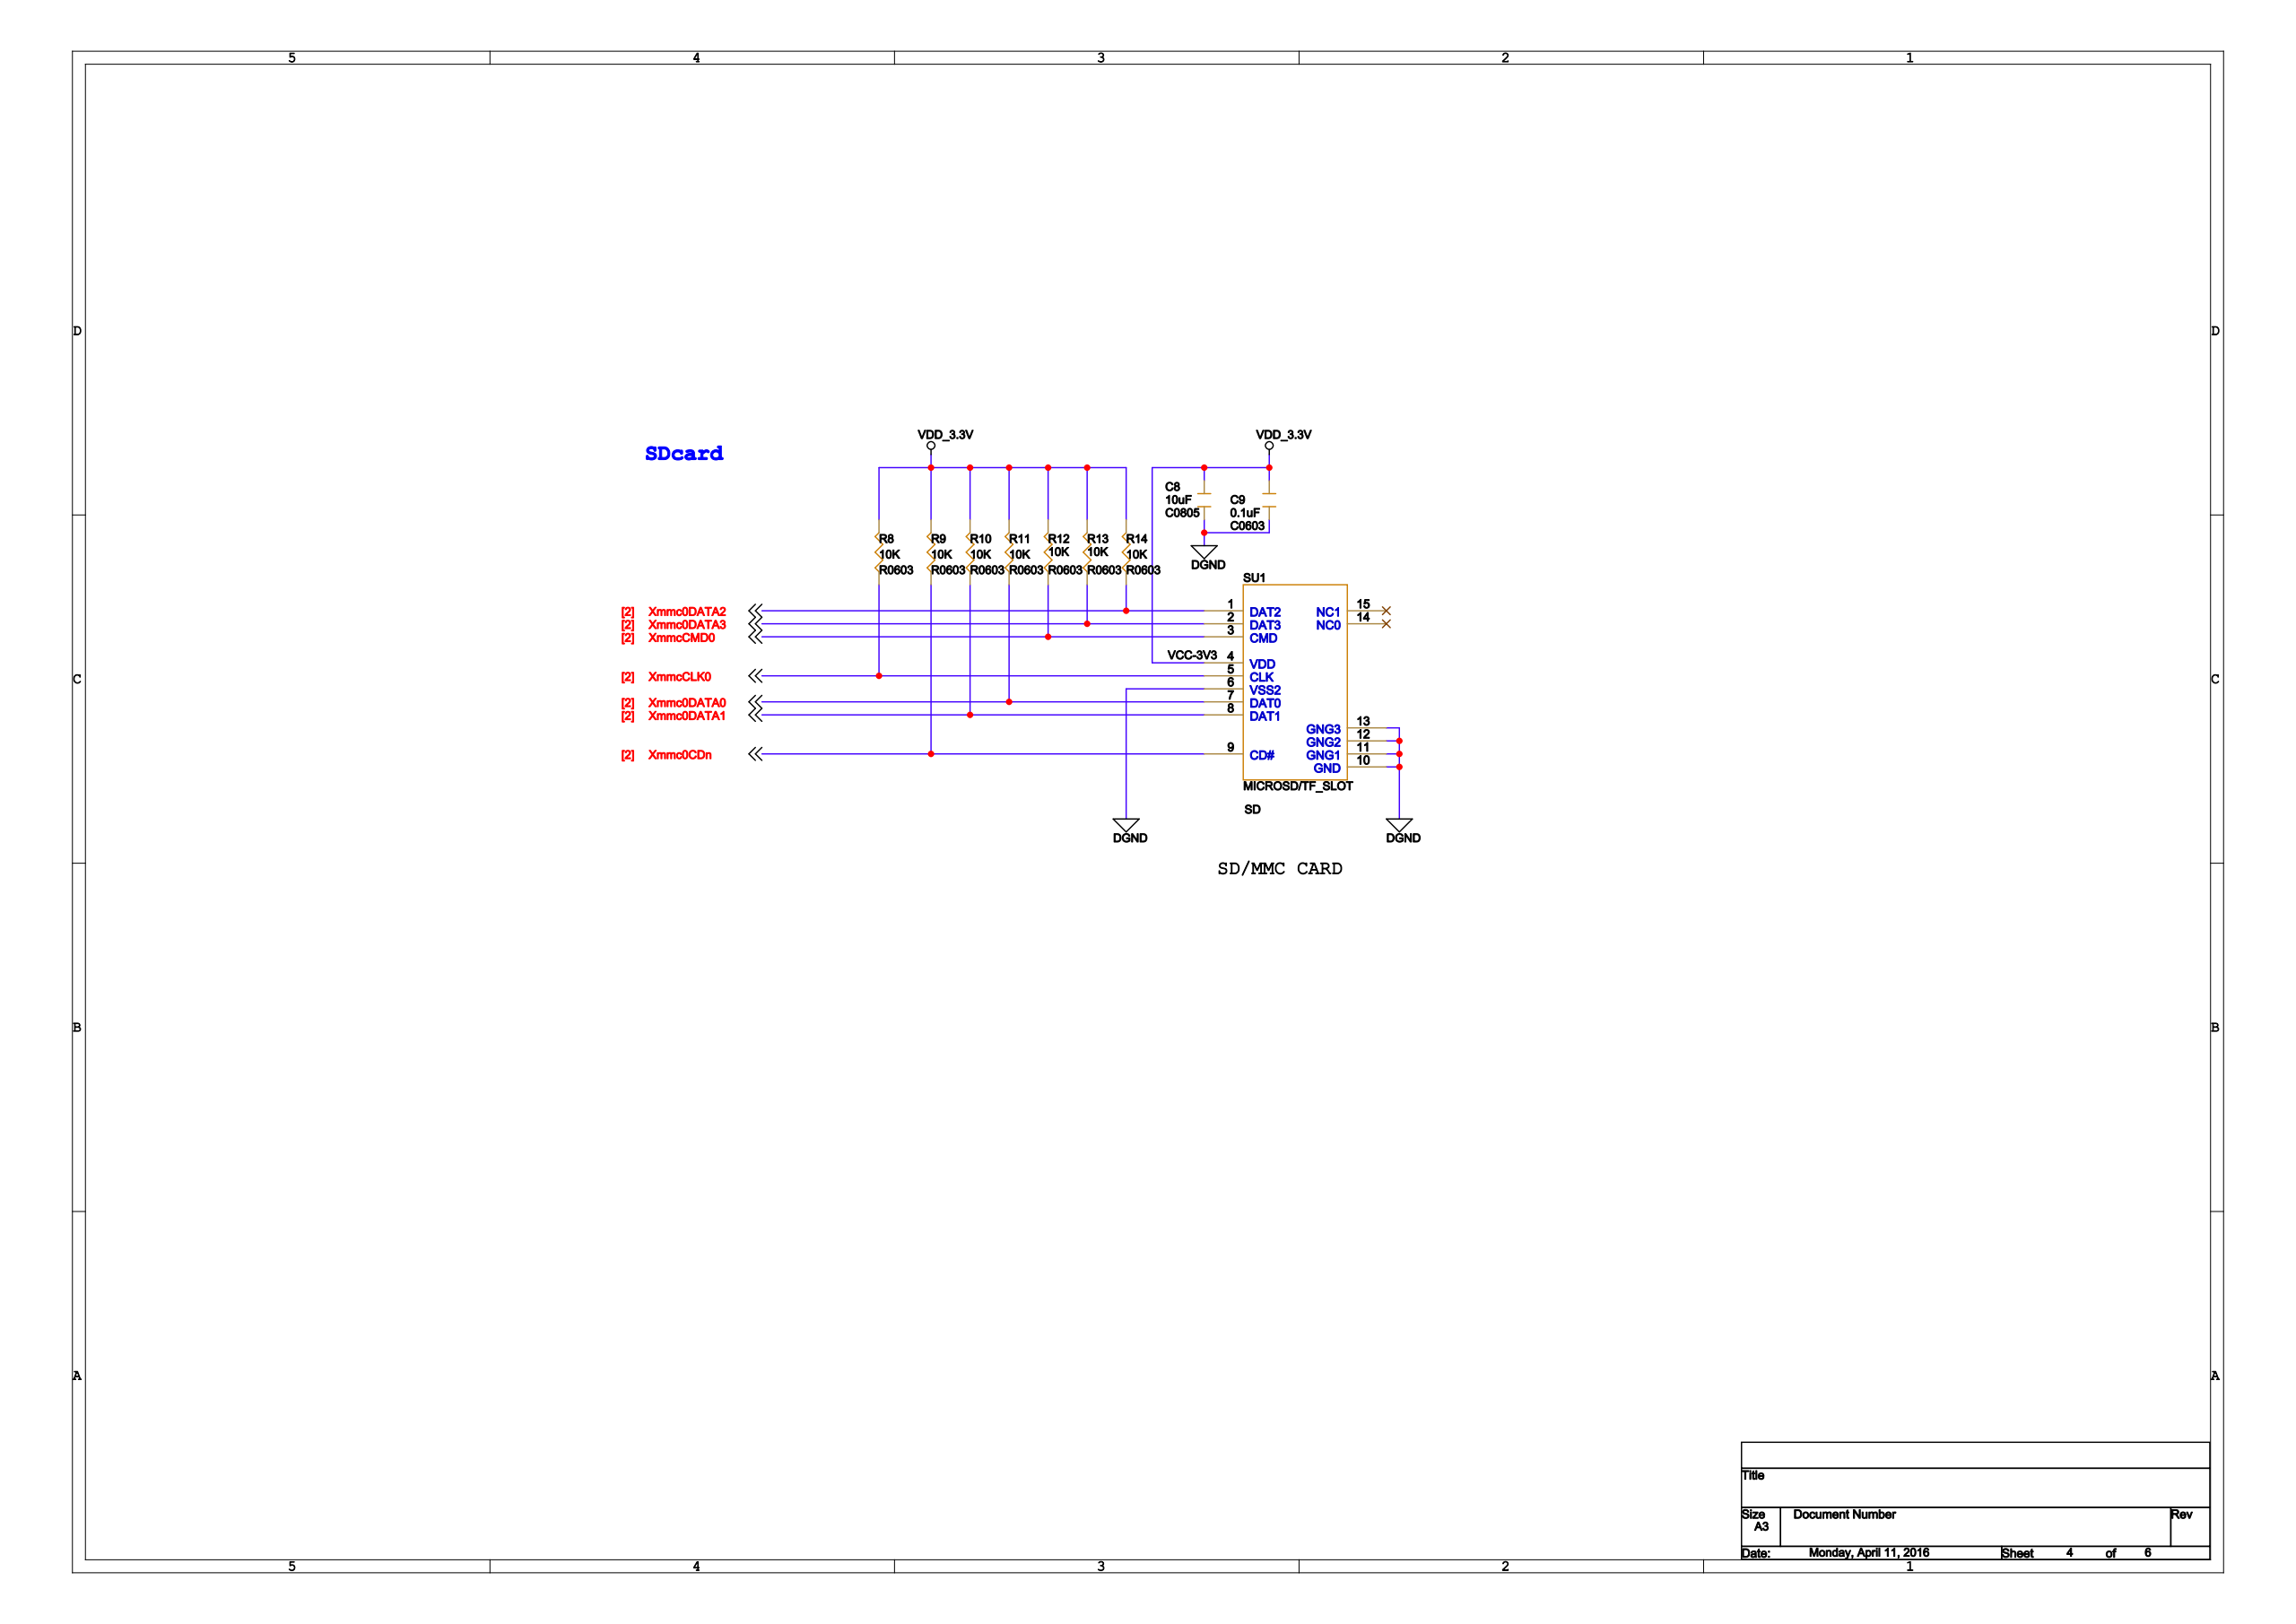Circuit board | Cadence Allegro | 85 parts | 48 nets | one sheet of the schematic
Parts on this sheet (reference | value | footprint):
C8 | 10uF | C0805
C9 | 0.1uF | C0603
R8 | 10K | R0603
R9 | 10K | R0603
R10 | 10K | R0603
R11 | 10K | R0603
R12 | 10K | R0603
R13 | 10K | R0603
R14 | 10K | R0603
SU1 | MICROSD/TF_SLOT | SD
Nets of these parts (net: part-pin ...):
DGND: C8-1 C9-1 SU1-6 SU1-10 SU1-11 SU1-12 SU1-13
VDD_3.3V: C8-2 C9-2 R8-2 R9-2 R10-2 R11-2 R12-2 R13-2 R14-2 SU1-4
XMMC0DATA0: R11-1 SU1-7
XMMC0DATA1: R10-1 SU1-8
XMMC0DATA2: R14-1 SU1-1
XMMC0DATA3: R13-1 SU1-2
XMMC0CDN: R9-1 SU1-9
XMMCCMD0: R12-1 SU1-3
XMMCCLK0: R8-1 SU1-5